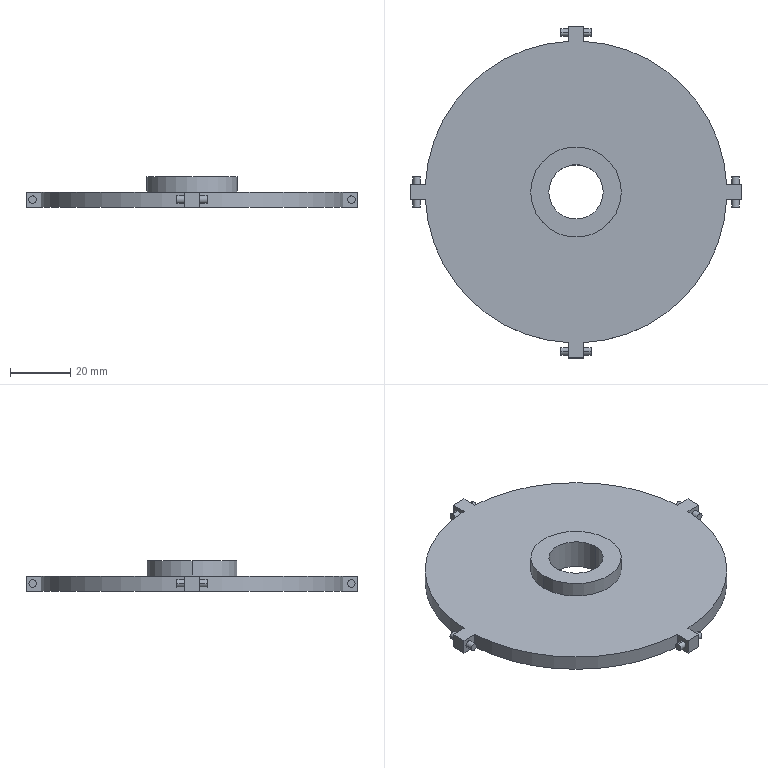Part | SolidWorks | features ICE 4, CirPattern 1, Extrusion 1 | 1 solid | 47 faces | box 110 x 110 x 10 mm | volume 40860 mm3 | cylinder 24 | plane 23 | commonest cylinder face diameters 2.5 x16 100 x4 18 x2 30 x2
STEP:
#1=CARTESIAN_POINT('',(54.05,-5.,2.5));
#2=VERTEX_POINT('',#1);
#3=CARTESIAN_POINT('',(51.55,-5.,2.5));
#4=VERTEX_POINT('',#3);
#5=CARTESIAN_POINT('',(52.8,-5.,2.5));
#6=DIRECTION('',(0.,-1.,0.));
#7=DIRECTION('',(0.,0.,-1.));
#8=AXIS2_PLACEMENT_3D('',#5,#6,#7);
#9=CIRCLE('',#8,1.25);
#10=EDGE_CURVE('',#2,#4,#9,.T.);
#11=ORIENTED_EDGE('',*,*,#10,.F.);
#12=CARTESIAN_POINT('',(54.05,-2.5,2.5));
#13=VERTEX_POINT('',#12);
#14=CARTESIAN_POINT('',(54.05,-5.,2.5));
#15=DIRECTION('',(0.,1.,0.));
#16=VECTOR('',#15,1000.);
#17=LINE('',#14,#16);
#18=EDGE_CURVE('',#2,#13,#17,.T.);
#19=ORIENTED_EDGE('',*,*,#18,.T.);
#20=CARTESIAN_POINT('',(51.55,-2.5,2.5));
#21=VERTEX_POINT('',#20);
#22=CARTESIAN_POINT('',(52.8,-2.5,2.5));
#23=DIRECTION('',(0.,1.,0.));
#24=DIRECTION('',(1.,0.,0.));
#25=AXIS2_PLACEMENT_3D('',#22,#23,#24);
#26=CIRCLE('',#25,1.25);
#27=EDGE_CURVE('',#21,#13,#26,.T.);
#28=ORIENTED_EDGE('',*,*,#27,.F.);
#29=CARTESIAN_POINT('',(51.55,-5.,2.5));
#30=DIRECTION('',(0.,1.,0.));
#31=VECTOR('',#30,1000.);
#32=LINE('',#29,#31);
#33=EDGE_CURVE('',#4,#21,#32,.T.);
#34=ORIENTED_EDGE('',*,*,#33,.F.);
#35=EDGE_LOOP('',(#11,#19,#28,#34));
#36=FACE_OUTER_BOUND('',#35,.T.);
#37=CARTESIAN_POINT('',(52.8,-5.,2.5));
#38=DIRECTION('',(0.,1.,0.));
#39=DIRECTION('',(-1.,0.,0.));
#40=AXIS2_PLACEMENT_3D('',#37,#38,#39);
#41=CYLINDRICAL_SURFACE('',#40,1.25);
#42=ADVANCED_FACE('',(#36),#41,.T.);
#43=CARTESIAN_POINT('',(54.05,2.5,2.5));
#44=VERTEX_POINT('',#43);
#45=CARTESIAN_POINT('',(51.55,2.5,2.5));
#46=VERTEX_POINT('',#45);
#47=CARTESIAN_POINT('',(52.8,2.5,2.5));
#48=DIRECTION('',(0.,-1.,0.));
#49=DIRECTION('',(-1.,0.,0.));
#50=AXIS2_PLACEMENT_3D('',#47,#48,#49);
#51=CIRCLE('',#50,1.25);
#52=EDGE_CURVE('',#44,#46,#51,.T.);
#53=ORIENTED_EDGE('',*,*,#52,.F.);
#54=CARTESIAN_POINT('',(54.05,5.,2.5));
#55=VERTEX_POINT('',#54);
#56=CARTESIAN_POINT('',(54.05,-5.,2.5));
#57=DIRECTION('',(0.,1.,0.));
#58=VECTOR('',#57,1000.);
#59=LINE('',#56,#58);
#60=EDGE_CURVE('',#44,#55,#59,.T.);
#61=ORIENTED_EDGE('',*,*,#60,.T.);
#62=CARTESIAN_POINT('',(51.55,5.,2.5));
#63=VERTEX_POINT('',#62);
#64=CARTESIAN_POINT('',(52.8,5.,2.5));
#65=DIRECTION('',(0.,-1.,0.));
#66=DIRECTION('',(0.,0.,-1.));
#67=AXIS2_PLACEMENT_3D('',#64,#65,#66);
#68=CIRCLE('',#67,1.25);
#69=EDGE_CURVE('',#55,#63,#68,.T.);
#70=ORIENTED_EDGE('',*,*,#69,.T.);
#71=CARTESIAN_POINT('',(51.55,-5.,2.5));
#72=DIRECTION('',(0.,1.,0.));
#73=VECTOR('',#72,1000.);
#74=LINE('',#71,#73);
#75=EDGE_CURVE('',#46,#63,#74,.T.);
#76=ORIENTED_EDGE('',*,*,#75,.F.);
#77=EDGE_LOOP('',(#53,#61,#70,#76));
#78=FACE_OUTER_BOUND('',#77,.T.);
#79=CARTESIAN_POINT('',(52.8,-5.,2.5));
#80=DIRECTION('',(0.,1.,0.));
#81=DIRECTION('',(-1.,0.,0.));
#82=AXIS2_PLACEMENT_3D('',#79,#80,#81);
#83=CYLINDRICAL_SURFACE('',#82,1.25);
#84=ADVANCED_FACE('',(#78),#83,.T.);
#85=CARTESIAN_POINT('',(2.5,-52.8,3.75));
#86=VERTEX_POINT('',#85);
#87=CARTESIAN_POINT('',(2.5,-52.8,1.25));
#88=VERTEX_POINT('',#87);
#89=CARTESIAN_POINT('',(2.5,-52.8,2.5));
#90=DIRECTION('',(-1.,0.,0.));
#91=DIRECTION('',(0.,0.,-1.));
#92=AXIS2_PLACEMENT_3D('',#89,#90,#91);
#93=CIRCLE('',#92,1.25);
#94=EDGE_CURVE('',#86,#88,#93,.T.);
#95=ORIENTED_EDGE('',*,*,#94,.F.);
#96=CARTESIAN_POINT('',(5.,-52.8,3.75));
#97=VERTEX_POINT('',#96);
#98=CARTESIAN_POINT('',(-5.,-52.8,3.75));
#99=DIRECTION('',(1.,0.,0.));
#100=VECTOR('',#99,1000.);
#101=LINE('',#98,#100);
#102=EDGE_CURVE('',#86,#97,#101,.T.);
#103=ORIENTED_EDGE('',*,*,#102,.T.);
#104=CARTESIAN_POINT('',(5.,-52.8,1.25));
#105=VERTEX_POINT('',#104);
#106=CARTESIAN_POINT('',(5.,-52.8,2.5));
#107=DIRECTION('',(-1.,0.,0.));
#108=DIRECTION('',(0.,0.,-1.));
#109=AXIS2_PLACEMENT_3D('',#106,#107,#108);
#110=CIRCLE('',#109,1.25);
#111=EDGE_CURVE('',#97,#105,#110,.T.);
#112=ORIENTED_EDGE('',*,*,#111,.T.);
#113=CARTESIAN_POINT('',(-5.,-52.8,1.25));
#114=DIRECTION('',(1.,0.,0.));
#115=VECTOR('',#114,1000.);
#116=LINE('',#113,#115);
#117=EDGE_CURVE('',#88,#105,#116,.T.);
#118=ORIENTED_EDGE('',*,*,#117,.F.);
#119=EDGE_LOOP('',(#95,#103,#112,#118));
#120=FACE_OUTER_BOUND('',#119,.T.);
#121=CARTESIAN_POINT('',(-5.,-52.8,2.5));
#122=DIRECTION('',(1.,0.,0.));
#123=DIRECTION('',(0.,0.,-1.));
#124=AXIS2_PLACEMENT_3D('',#121,#122,#123);
#125=CYLINDRICAL_SURFACE('',#124,1.25);
#126=ADVANCED_FACE('',(#120),#125,.T.);
#127=CARTESIAN_POINT('',(-5.,-52.8,3.75));
#128=VERTEX_POINT('',#127);
#129=CARTESIAN_POINT('',(-5.,-52.8,1.25));
#130=VERTEX_POINT('',#129);
#131=CARTESIAN_POINT('',(-5.,-52.8,2.5));
#132=DIRECTION('',(-1.,0.,0.));
#133=DIRECTION('',(0.,0.,-1.));
#134=AXIS2_PLACEMENT_3D('',#131,#132,#133);
#135=CIRCLE('',#134,1.25);
#136=EDGE_CURVE('',#128,#130,#135,.T.);
#137=ORIENTED_EDGE('',*,*,#136,.F.);
#138=CARTESIAN_POINT('',(-2.5,-52.8,3.75));
#139=VERTEX_POINT('',#138);
#140=CARTESIAN_POINT('',(-5.,-52.8,3.75));
#141=DIRECTION('',(1.,0.,0.));
#142=VECTOR('',#141,1000.);
#143=LINE('',#140,#142);
#144=EDGE_CURVE('',#128,#139,#143,.T.);
#145=ORIENTED_EDGE('',*,*,#144,.T.);
#146=CARTESIAN_POINT('',(-2.5,-52.8,1.25));
#147=VERTEX_POINT('',#146);
#148=CARTESIAN_POINT('',(-2.5,-52.8,2.5));
#149=DIRECTION('',(1.,0.,0.));
#150=DIRECTION('',(0.,0.,1.));
#151=AXIS2_PLACEMENT_3D('',#148,#149,#150);
#152=CIRCLE('',#151,1.25);
#153=EDGE_CURVE('',#147,#139,#152,.T.);
#154=ORIENTED_EDGE('',*,*,#153,.F.);
#155=CARTESIAN_POINT('',(-5.,-52.8,1.25));
#156=DIRECTION('',(1.,0.,0.));
#157=VECTOR('',#156,1000.);
#158=LINE('',#155,#157);
#159=EDGE_CURVE('',#130,#147,#158,.T.);
#160=ORIENTED_EDGE('',*,*,#159,.F.);
#161=EDGE_LOOP('',(#137,#145,#154,#160));
#162=FACE_OUTER_BOUND('',#161,.T.);
#163=CARTESIAN_POINT('',(-5.,-52.8,2.5));
#164=DIRECTION('',(1.,0.,0.));
#165=DIRECTION('',(0.,0.,-1.));
#166=AXIS2_PLACEMENT_3D('',#163,#164,#165);
#167=CYLINDRICAL_SURFACE('',#166,1.25);
#168=ADVANCED_FACE('',(#162),#167,.T.);
#169=CARTESIAN_POINT('',(-54.05,5.,2.5));
#170=VERTEX_POINT('',#169);
#171=CARTESIAN_POINT('',(-51.55,5.,2.5));
#172=VERTEX_POINT('',#171);
#173=CARTESIAN_POINT('',(-52.8,5.,2.5));
#174=DIRECTION('',(0.,1.,0.));
#175=DIRECTION('',(0.,0.,-1.));
#176=AXIS2_PLACEMENT_3D('',#173,#174,#175);
#177=CIRCLE('',#176,1.25);
#178=EDGE_CURVE('',#170,#172,#177,.T.);
#179=ORIENTED_EDGE('',*,*,#178,.F.);
#180=CARTESIAN_POINT('',(-54.05,2.5,2.5));
#181=VERTEX_POINT('',#180);
#182=CARTESIAN_POINT('',(-54.05,5.,2.5));
#183=DIRECTION('',(0.,-1.,0.));
#184=VECTOR('',#183,1000.);
#185=LINE('',#182,#184);
#186=EDGE_CURVE('',#170,#181,#185,.T.);
#187=ORIENTED_EDGE('',*,*,#186,.T.);
#188=CARTESIAN_POINT('',(-51.55,2.5,2.5));
#189=VERTEX_POINT('',#188);
#190=CARTESIAN_POINT('',(-52.8,2.5,2.5));
#191=DIRECTION('',(0.,-1.,0.));
#192=DIRECTION('',(-1.,0.,0.));
#193=AXIS2_PLACEMENT_3D('',#190,#191,#192);
#194=CIRCLE('',#193,1.25);
#195=EDGE_CURVE('',#189,#181,#194,.T.);
#196=ORIENTED_EDGE('',*,*,#195,.F.);
#197=CARTESIAN_POINT('',(-51.55,5.,2.5));
#198=DIRECTION('',(0.,-1.,0.));
#199=VECTOR('',#198,1000.);
#200=LINE('',#197,#199);
#201=EDGE_CURVE('',#172,#189,#200,.T.);
#202=ORIENTED_EDGE('',*,*,#201,.F.);
#203=EDGE_LOOP('',(#179,#187,#196,#202));
#204=FACE_OUTER_BOUND('',#203,.T.);
#205=CARTESIAN_POINT('',(-52.8,5.,2.5));
#206=DIRECTION('',(0.,-1.,0.));
#207=DIRECTION('',(1.,0.,0.));
#208=AXIS2_PLACEMENT_3D('',#205,#206,#207);
#209=CYLINDRICAL_SURFACE('',#208,1.25);
#210=ADVANCED_FACE('',(#204),#209,.T.);
#211=CARTESIAN_POINT('',(-54.05,-2.5,2.5));
#212=VERTEX_POINT('',#211);
#213=CARTESIAN_POINT('',(-51.55,-2.5,2.5));
#214=VERTEX_POINT('',#213);
#215=CARTESIAN_POINT('',(-52.8,-2.5,2.5));
#216=DIRECTION('',(0.,1.,0.));
#217=DIRECTION('',(1.,0.,0.));
#218=AXIS2_PLACEMENT_3D('',#215,#216,#217);
#219=CIRCLE('',#218,1.25);
#220=EDGE_CURVE('',#212,#214,#219,.T.);
#221=ORIENTED_EDGE('',*,*,#220,.F.);
#222=CARTESIAN_POINT('',(-54.05,-5.,2.5));
#223=VERTEX_POINT('',#222);
#224=CARTESIAN_POINT('',(-54.05,5.,2.5));
#225=DIRECTION('',(0.,-1.,0.));
#226=VECTOR('',#225,1000.);
#227=LINE('',#224,#226);
#228=EDGE_CURVE('',#212,#223,#227,.T.);
#229=ORIENTED_EDGE('',*,*,#228,.T.);
#230=CARTESIAN_POINT('',(-51.55,-5.,2.5));
#231=VERTEX_POINT('',#230);
#232=CARTESIAN_POINT('',(-52.8,-5.,2.5));
#233=DIRECTION('',(0.,1.,0.));
#234=DIRECTION('',(0.,0.,-1.));
#235=AXIS2_PLACEMENT_3D('',#232,#233,#234);
#236=CIRCLE('',#235,1.25);
#237=EDGE_CURVE('',#223,#231,#236,.T.);
#238=ORIENTED_EDGE('',*,*,#237,.T.);
#239=CARTESIAN_POINT('',(-51.55,5.,2.5));
#240=DIRECTION('',(0.,-1.,0.));
#241=VECTOR('',#240,1000.);
#242=LINE('',#239,#241);
#243=EDGE_CURVE('',#214,#231,#242,.T.);
#244=ORIENTED_EDGE('',*,*,#243,.F.);
#245=EDGE_LOOP('',(#221,#229,#238,#244));
#246=FACE_OUTER_BOUND('',#245,.T.);
#247=CARTESIAN_POINT('',(-52.8,5.,2.5));
#248=DIRECTION('',(0.,-1.,0.));
#249=DIRECTION('',(1.,0.,0.));
#250=AXIS2_PLACEMENT_3D('',#247,#248,#249);
#251=CYLINDRICAL_SURFACE('',#250,1.25);
#252=ADVANCED_FACE('',(#246),#251,.T.);
#253=CARTESIAN_POINT('',(5.,52.8,1.25));
#254=VERTEX_POINT('',#253);
#255=CARTESIAN_POINT('',(5.,52.8,3.75));
#256=VERTEX_POINT('',#255);
#257=CARTESIAN_POINT('',(5.,52.8,2.5));
#258=DIRECTION('',(1.,0.,0.));
#259=DIRECTION('',(0.,0.,-1.));
#260=AXIS2_PLACEMENT_3D('',#257,#258,#259);
#261=CIRCLE('',#260,1.25);
#262=EDGE_CURVE('',#254,#256,#261,.T.);
#263=ORIENTED_EDGE('',*,*,#262,.F.);
#264=CARTESIAN_POINT('',(2.5,52.8,1.25));
#265=VERTEX_POINT('',#264);
#266=CARTESIAN_POINT('',(5.,52.8,1.25));
#267=DIRECTION('',(-1.,0.,0.));
#268=VECTOR('',#267,1000.);
#269=LINE('',#266,#268);
#270=EDGE_CURVE('',#254,#265,#269,.T.);
#271=ORIENTED_EDGE('',*,*,#270,.T.);
#272=CARTESIAN_POINT('',(2.5,52.8,3.75));
#273=VERTEX_POINT('',#272);
#274=CARTESIAN_POINT('',(2.5,52.8,2.5));
#275=DIRECTION('',(-1.,0.,0.));
#276=DIRECTION('',(0.,0.,-1.));
#277=AXIS2_PLACEMENT_3D('',#274,#275,#276);
#278=CIRCLE('',#277,1.25);
#279=EDGE_CURVE('',#273,#265,#278,.T.);
#280=ORIENTED_EDGE('',*,*,#279,.F.);
#281=CARTESIAN_POINT('',(5.,52.8,3.75));
#282=DIRECTION('',(-1.,0.,0.));
#283=VECTOR('',#282,1000.);
#284=LINE('',#281,#283);
#285=EDGE_CURVE('',#256,#273,#284,.T.);
#286=ORIENTED_EDGE('',*,*,#285,.F.);
#287=EDGE_LOOP('',(#263,#271,#280,#286));
#288=FACE_OUTER_BOUND('',#287,.T.);
#289=CARTESIAN_POINT('',(5.,52.8,2.5));
#290=DIRECTION('',(-1.,0.,0.));
#291=DIRECTION('',(0.,0.,1.));
#292=AXIS2_PLACEMENT_3D('',#289,#290,#291);
#293=CYLINDRICAL_SURFACE('',#292,1.25);
#294=ADVANCED_FACE('',(#288),#293,.T.);
#295=CARTESIAN_POINT('',(-2.5,52.8,1.25));
#296=VERTEX_POINT('',#295);
#297=CARTESIAN_POINT('',(-2.5,52.8,3.75));
#298=VERTEX_POINT('',#297);
#299=CARTESIAN_POINT('',(-2.5,52.8,2.5));
#300=DIRECTION('',(1.,0.,0.));
#301=DIRECTION('',(0.,0.,1.));
#302=AXIS2_PLACEMENT_3D('',#299,#300,#301);
#303=CIRCLE('',#302,1.25);
#304=EDGE_CURVE('',#296,#298,#303,.T.);
#305=ORIENTED_EDGE('',*,*,#304,.F.);
#306=CARTESIAN_POINT('',(-5.,52.8,1.25));
#307=VERTEX_POINT('',#306);
#308=CARTESIAN_POINT('',(5.,52.8,1.25));
#309=DIRECTION('',(-1.,0.,0.));
#310=VECTOR('',#309,1000.);
#311=LINE('',#308,#310);
#312=EDGE_CURVE('',#296,#307,#311,.T.);
#313=ORIENTED_EDGE('',*,*,#312,.T.);
#314=CARTESIAN_POINT('',(-5.,52.8,3.75));
#315=VERTEX_POINT('',#314);
#316=CARTESIAN_POINT('',(-5.,52.8,2.5));
#317=DIRECTION('',(1.,0.,0.));
#318=DIRECTION('',(0.,0.,-1.));
#319=AXIS2_PLACEMENT_3D('',#316,#317,#318);
#320=CIRCLE('',#319,1.25);
#321=EDGE_CURVE('',#307,#315,#320,.T.);
#322=ORIENTED_EDGE('',*,*,#321,.T.);
#323=CARTESIAN_POINT('',(5.,52.8,3.75));
#324=DIRECTION('',(-1.,0.,0.));
#325=VECTOR('',#324,1000.);
#326=LINE('',#323,#325);
#327=EDGE_CURVE('',#298,#315,#326,.T.);
#328=ORIENTED_EDGE('',*,*,#327,.F.);
#329=EDGE_LOOP('',(#305,#313,#322,#328));
#330=FACE_OUTER_BOUND('',#329,.T.);
#331=CARTESIAN_POINT('',(5.,52.8,2.5));
#332=DIRECTION('',(-1.,0.,0.));
#333=DIRECTION('',(0.,0.,1.));
#334=AXIS2_PLACEMENT_3D('',#331,#332,#333);
#335=CYLINDRICAL_SURFACE('',#334,1.25);
#336=ADVANCED_FACE('',(#330),#335,.T.);
#337=CARTESIAN_POINT('',(-9.,0.,0.));
#338=VERTEX_POINT('',#337);
#339=CARTESIAN_POINT('',(9.,0.,0.));
#340=VERTEX_POINT('',#339);
#341=CARTESIAN_POINT('',(0.,0.,0.));
#342=DIRECTION('',(0.,0.,1.));
#343=DIRECTION('',(1.,0.,0.));
#344=AXIS2_PLACEMENT_3D('',#341,#342,#343);
#345=CIRCLE('',#344,9.);
#346=EDGE_CURVE('',#338,#340,#345,.T.);
#347=ORIENTED_EDGE('',*,*,#346,.F.);
#348=CARTESIAN_POINT('',(-9.,0.,10.));
#349=VERTEX_POINT('',#348);
#350=CARTESIAN_POINT('',(-9.,0.,-5.));
#351=DIRECTION('',(0.,0.,1.));
#352=VECTOR('',#351,1000.);
#353=LINE('',#350,#352);
#354=EDGE_CURVE('',#338,#349,#353,.T.);
#355=ORIENTED_EDGE('',*,*,#354,.T.);
#356=CARTESIAN_POINT('',(9.,0.,10.));
#357=VERTEX_POINT('',#356);
#358=CARTESIAN_POINT('',(0.,0.,10.));
#359=DIRECTION('',(0.,0.,1.));
#360=DIRECTION('',(1.,0.,0.));
#361=AXIS2_PLACEMENT_3D('',#358,#359,#360);
#362=CIRCLE('',#361,9.);
#363=EDGE_CURVE('',#349,#357,#362,.T.);
#364=ORIENTED_EDGE('',*,*,#363,.T.);
#365=CARTESIAN_POINT('',(9.,0.,-5.));
#366=DIRECTION('',(0.,0.,1.));
#367=VECTOR('',#366,1000.);
#368=LINE('',#365,#367);
#369=EDGE_CURVE('',#340,#357,#368,.T.);
#370=ORIENTED_EDGE('',*,*,#369,.F.);
#371=EDGE_LOOP('',(#347,#355,#364,#370));
#372=FACE_OUTER_BOUND('',#371,.T.);
#373=CARTESIAN_POINT('',(0.,0.,-5.));
#374=DIRECTION('',(0.,0.,1.));
#375=DIRECTION('',(1.,0.,0.));
#376=AXIS2_PLACEMENT_3D('',#373,#374,#375);
#377=CYLINDRICAL_SURFACE('',#376,9.);
#378=ADVANCED_FACE('',(#372),#377,.F.);
#379=CARTESIAN_POINT('',(15.,0.,10.));
#380=VERTEX_POINT('',#379);
#381=CARTESIAN_POINT('',(-15.,0.,10.));
#382=VERTEX_POINT('',#381);
#383=CARTESIAN_POINT('',(0.,0.,10.));
#384=DIRECTION('',(0.,0.,1.));
#385=DIRECTION('',(1.,0.,0.));
#386=AXIS2_PLACEMENT_3D('',#383,#384,#385);
#387=CIRCLE('',#386,15.);
#388=EDGE_CURVE('',#380,#382,#387,.T.);
#389=ORIENTED_EDGE('',*,*,#388,.F.);
#390=CARTESIAN_POINT('',(15.,0.,5.));
#391=VERTEX_POINT('',#390);
#392=CARTESIAN_POINT('',(15.,0.,10.));
#393=DIRECTION('',(0.,0.,-1.));
#394=VECTOR('',#393,1000.);
#395=LINE('',#392,#394);
#396=EDGE_CURVE('',#380,#391,#395,.T.);
#397=ORIENTED_EDGE('',*,*,#396,.T.);
#398=CARTESIAN_POINT('',(-15.,0.,5.));
#399=VERTEX_POINT('',#398);
#400=CARTESIAN_POINT('',(0.,0.,5.));
#401=DIRECTION('',(0.,0.,1.));
#402=DIRECTION('',(1.,0.,0.));
#403=AXIS2_PLACEMENT_3D('',#400,#401,#402);
#404=CIRCLE('',#403,15.);
#405=EDGE_CURVE('',#391,#399,#404,.T.);
#406=ORIENTED_EDGE('',*,*,#405,.T.);
#407=CARTESIAN_POINT('',(-15.,0.,10.));
#408=DIRECTION('',(0.,0.,-1.));
#409=VECTOR('',#408,1000.);
#410=LINE('',#407,#409);
#411=EDGE_CURVE('',#382,#399,#410,.T.);
#412=ORIENTED_EDGE('',*,*,#411,.F.);
#413=EDGE_LOOP('',(#389,#397,#406,#412));
#414=FACE_OUTER_BOUND('',#413,.T.);
#415=CARTESIAN_POINT('',(0.,0.,10.));
#416=DIRECTION('',(0.,0.,-1.));
#417=DIRECTION('',(-1.,0.,0.));
#418=AXIS2_PLACEMENT_3D('',#415,#416,#417);
#419=CYLINDRICAL_SURFACE('',#418,15.);
#420=ADVANCED_FACE('',(#414),#419,.T.);
#421=CARTESIAN_POINT('',(2.5,-49.937,0.));
#422=VERTEX_POINT('',#421);
#423=CARTESIAN_POINT('',(49.937,-2.5,0.));
#424=VERTEX_POINT('',#423);
#425=CARTESIAN_POINT('',(0.,0.,0.));
#426=DIRECTION('',(0.,0.,1.));
#427=DIRECTION('',(1.,0.,0.));
#428=AXIS2_PLACEMENT_3D('',#425,#426,#427);
#429=CIRCLE('',#428,50.);
#430=EDGE_CURVE('',#422,#424,#429,.T.);
#431=ORIENTED_EDGE('',*,*,#430,.T.);
#432=CARTESIAN_POINT('',(49.937,-2.5,5.));
#433=VERTEX_POINT('',#432);
#434=CARTESIAN_POINT('',(49.937,-2.5,5.));
#435=DIRECTION('',(0.,0.,-1.));
#436=VECTOR('',#435,1000.);
#437=LINE('',#434,#436);
#438=EDGE_CURVE('',#433,#424,#437,.T.);
#439=ORIENTED_EDGE('',*,*,#438,.F.);
#440=CARTESIAN_POINT('',(2.5,-49.937,5.));
#441=VERTEX_POINT('',#440);
#442=CARTESIAN_POINT('',(0.,0.,5.));
#443=DIRECTION('',(0.,0.,1.));
#444=DIRECTION('',(1.,0.,0.));
#445=AXIS2_PLACEMENT_3D('',#442,#443,#444);
#446=CIRCLE('',#445,50.);
#447=EDGE_CURVE('',#441,#433,#446,.T.);
#448=ORIENTED_EDGE('',*,*,#447,.F.);
#449=CARTESIAN_POINT('',(2.5,-49.937,5.));
#450=DIRECTION('',(0.,0.,1.));
#451=VECTOR('',#450,1000.);
#452=LINE('',#449,#451);
#453=EDGE_CURVE('',#422,#441,#452,.T.);
#454=ORIENTED_EDGE('',*,*,#453,.F.);
#455=EDGE_LOOP('',(#431,#439,#448,#454));
#456=FACE_OUTER_BOUND('',#455,.T.);
#457=CARTESIAN_POINT('',(0.,0.,5.));
#458=DIRECTION('',(0.,0.,-1.));
#459=DIRECTION('',(-1.,0.,0.));
#460=AXIS2_PLACEMENT_3D('',#457,#458,#459);
#461=CYLINDRICAL_SURFACE('',#460,50.);
#462=ADVANCED_FACE('',(#456),#461,.T.);
#463=CARTESIAN_POINT('',(49.937,2.5,5.));
#464=VERTEX_POINT('',#463);
#465=CARTESIAN_POINT('',(2.5,49.937,5.));
#466=VERTEX_POINT('',#465);
#467=CARTESIAN_POINT('',(0.,0.,5.));
#468=DIRECTION('',(0.,0.,1.));
#469=DIRECTION('',(1.,0.,0.));
#470=AXIS2_PLACEMENT_3D('',#467,#468,#469);
#471=CIRCLE('',#470,50.);
#472=EDGE_CURVE('',#464,#466,#471,.T.);
#473=ORIENTED_EDGE('',*,*,#472,.F.);
#474=CARTESIAN_POINT('',(49.937,2.5,0.));
#475=VERTEX_POINT('',#474);
#476=CARTESIAN_POINT('',(49.937,2.5,5.));
#477=DIRECTION('',(0.,0.,1.));
#478=VECTOR('',#477,1000.);
#479=LINE('',#476,#478);
#480=EDGE_CURVE('',#475,#464,#479,.T.);
#481=ORIENTED_EDGE('',*,*,#480,.F.);
#482=CARTESIAN_POINT('',(2.5,49.937,0.));
#483=VERTEX_POINT('',#482);
#484=CARTESIAN_POINT('',(0.,0.,0.));
#485=DIRECTION('',(0.,0.,1.));
#486=DIRECTION('',(1.,0.,0.));
#487=AXIS2_PLACEMENT_3D('',#484,#485,#486);
#488=CIRCLE('',#487,50.);
#489=EDGE_CURVE('',#475,#483,#488,.T.);
#490=ORIENTED_EDGE('',*,*,#489,.T.);
#491=CARTESIAN_POINT('',(2.5,49.937,5.));
#492=DIRECTION('',(0.,0.,-1.));
#493=VECTOR('',#492,1000.);
#494=LINE('',#491,#493);
#495=EDGE_CURVE('',#466,#483,#494,.T.);
#496=ORIENTED_EDGE('',*,*,#495,.F.);
#497=EDGE_LOOP('',(#473,#481,#490,#496));
#498=FACE_OUTER_BOUND('',#497,.T.);
#499=CARTESIAN_POINT('',(0.,0.,5.));
#500=DIRECTION('',(0.,0.,-1.));
#501=DIRECTION('',(-1.,0.,0.));
#502=AXIS2_PLACEMENT_3D('',#499,#500,#501);
#503=CYLINDRICAL_SURFACE('',#502,50.);
#504=ADVANCED_FACE('',(#498),#503,.T.);
#505=CARTESIAN_POINT('',(-2.5,49.937,0.));
#506=VERTEX_POINT('',#505);
#507=CARTESIAN_POINT('',(-49.937,2.5,0.));
#508=VERTEX_POINT('',#507);
#509=CARTESIAN_POINT('',(0.,0.,0.));
#510=DIRECTION('',(0.,0.,1.));
#511=DIRECTION('',(1.,0.,0.));
#512=AXIS2_PLACEMENT_3D('',#509,#510,#511);
#513=CIRCLE('',#512,50.);
#514=EDGE_CURVE('',#506,#508,#513,.T.);
#515=ORIENTED_EDGE('',*,*,#514,.T.);
#516=CARTESIAN_POINT('',(-49.937,2.5,5.));
#517=VERTEX_POINT('',#516);
#518=CARTESIAN_POINT('',(-49.937,2.5,5.));
#519=DIRECTION('',(0.,0.,-1.));
#520=VECTOR('',#519,1000.);
#521=LINE('',#518,#520);
#522=EDGE_CURVE('',#517,#508,#521,.T.);
#523=ORIENTED_EDGE('',*,*,#522,.F.);
#524=CARTESIAN_POINT('',(-2.5,49.937,5.));
#525=VERTEX_POINT('',#524);
#526=CARTESIAN_POINT('',(0.,0.,5.));
#527=DIRECTION('',(0.,0.,1.));
#528=DIRECTION('',(1.,0.,0.));
#529=AXIS2_PLACEMENT_3D('',#526,#527,#528);
#530=CIRCLE('',#529,50.);
#531=EDGE_CURVE('',#525,#517,#530,.T.);
#532=ORIENTED_EDGE('',*,*,#531,.F.);
#533=CARTESIAN_POINT('',(-2.5,49.937,5.));
#534=DIRECTION('',(0.,0.,1.));
#535=VECTOR('',#534,1000.);
#536=LINE('',#533,#535);
#537=EDGE_CURVE('',#506,#525,#536,.T.);
#538=ORIENTED_EDGE('',*,*,#537,.F.);
#539=EDGE_LOOP('',(#515,#523,#532,#538));
#540=FACE_OUTER_BOUND('',#539,.T.);
#541=CARTESIAN_POINT('',(0.,0.,5.));
#542=DIRECTION('',(0.,0.,-1.));
#543=DIRECTION('',(-1.,0.,0.));
#544=AXIS2_PLACEMENT_3D('',#541,#542,#543);
#545=CYLINDRICAL_SURFACE('',#544,50.);
#546=ADVANCED_FACE('',(#540),#545,.T.);
#547=CARTESIAN_POINT('',(-49.937,-2.5,0.));
#548=VERTEX_POINT('',#547);
#549=CARTESIAN_POINT('',(-2.5,-49.937,0.));
#550=VERTEX_POINT('',#549);
#551=CARTESIAN_POINT('',(0.,0.,0.));
#552=DIRECTION('',(0.,0.,1.));
#553=DIRECTION('',(1.,0.,0.));
#554=AXIS2_PLACEMENT_3D('',#551,#552,#553);
#555=CIRCLE('',#554,50.);
#556=EDGE_CURVE('',#548,#550,#555,.T.);
#557=ORIENTED_EDGE('',*,*,#556,.T.);
#558=CARTESIAN_POINT('',(-2.5,-49.937,5.));
#559=VERTEX_POINT('',#558);
#560=CARTESIAN_POINT('',(-2.5,-49.937,5.));
#561=DIRECTION('',(0.,0.,-1.));
#562=VECTOR('',#561,1000.);
#563=LINE('',#560,#562);
#564=EDGE_CURVE('',#559,#550,#563,.T.);
#565=ORIENTED_EDGE('',*,*,#564,.F.);
#566=CARTESIAN_POINT('',(-49.937,-2.5,5.));
#567=VERTEX_POINT('',#566);
#568=CARTESIAN_POINT('',(0.,0.,5.));
#569=DIRECTION('',(0.,0.,1.));
#570=DIRECTION('',(1.,0.,0.));
#571=AXIS2_PLACEMENT_3D('',#568,#569,#570);
#572=CIRCLE('',#571,50.);
#573=EDGE_CURVE('',#567,#559,#572,.T.);
#574=ORIENTED_EDGE('',*,*,#573,.F.);
#575=CARTESIAN_POINT('',(-49.937,-2.5,5.));
#576=DIRECTION('',(0.,0.,1.));
#577=VECTOR('',#576,1000.);
#578=LINE('',#575,#577);
#579=EDGE_CURVE('',#548,#567,#578,.T.);
#580=ORIENTED_EDGE('',*,*,#579,.F.);
#581=EDGE_LOOP('',(#557,#565,#574,#580));
#582=FACE_OUTER_BOUND('',#581,.T.);
#583=CARTESIAN_POINT('',(0.,0.,5.));
#584=DIRECTION('',(0.,0.,-1.));
#585=DIRECTION('',(-1.,0.,0.));
#586=AXIS2_PLACEMENT_3D('',#583,#584,#585);
#587=CYLINDRICAL_SURFACE('',#586,50.);
#588=ADVANCED_FACE('',(#582),#587,.T.);
#589=CARTESIAN_POINT('',(0.,0.,5.));
#590=DIRECTION('',(0.,0.,1.));
#591=DIRECTION('',(1.,0.,0.));
#592=AXIS2_PLACEMENT_3D('',#589,#590,#591);
#593=CIRCLE('',#592,15.);
#594=EDGE_CURVE('',#399,#391,#593,.T.);
#595=ORIENTED_EDGE('',*,*,#594,.F.);
#596=ORIENTED_EDGE('',*,*,#405,.F.);
#597=EDGE_LOOP('',(#595,#596));
#598=FACE_BOUND('',#597,.T.);
#599=ORIENTED_EDGE('',*,*,#531,.T.);
#600=CARTESIAN_POINT('',(-55.,2.5,5.));
#601=VERTEX_POINT('',#600);
#602=CARTESIAN_POINT('',(50.001,2.5,5.));
#603=DIRECTION('',(-1.,0.,0.));
#604=VECTOR('',#603,1000.);
#605=LINE('',#602,#604);
#606=EDGE_CURVE('',#517,#601,#605,.T.);
#607=ORIENTED_EDGE('',*,*,#606,.T.);
#608=CARTESIAN_POINT('',(-55.,-2.5,5.));
#609=VERTEX_POINT('',#608);
#610=CARTESIAN_POINT('',(-55.,2.5,5.));
#611=DIRECTION('',(0.,1.,0.));
#612=VECTOR('',#611,1000.);
#613=LINE('',#610,#612);
#614=EDGE_CURVE('',#609,#601,#613,.T.);
#615=ORIENTED_EDGE('',*,*,#614,.F.);
#616=CARTESIAN_POINT('',(50.001,-2.5,5.));
#617=DIRECTION('',(-1.,0.,0.));
#618=VECTOR('',#617,1000.);
#619=LINE('',#616,#618);
#620=EDGE_CURVE('',#567,#609,#619,.T.);
#621=ORIENTED_EDGE('',*,*,#620,.F.);
#622=ORIENTED_EDGE('',*,*,#573,.T.);
#623=CARTESIAN_POINT('',(-2.5,-55.,5.));
#624=VERTEX_POINT('',#623);
#625=CARTESIAN_POINT('',(-2.5,55.001,5.));
#626=DIRECTION('',(0.,-1.,0.));
#627=VECTOR('',#626,1000.);
#628=LINE('',#625,#627);
#629=EDGE_CURVE('',#559,#624,#628,.T.);
#630=ORIENTED_EDGE('',*,*,#629,.T.);
#631=CARTESIAN_POINT('',(2.5,-55.,5.));
#632=VERTEX_POINT('',#631);
#633=CARTESIAN_POINT('',(-2.5,-55.,5.));
#634=DIRECTION('',(-1.,0.,0.));
#635=VECTOR('',#634,1000.);
#636=LINE('',#633,#635);
#637=EDGE_CURVE('',#632,#624,#636,.T.);
#638=ORIENTED_EDGE('',*,*,#637,.F.);
#639=CARTESIAN_POINT('',(2.5,55.001,5.));
#640=DIRECTION('',(0.,-1.,0.));
#641=VECTOR('',#640,1000.);
#642=LINE('',#639,#641);
#643=EDGE_CURVE('',#441,#632,#642,.T.);
#644=ORIENTED_EDGE('',*,*,#643,.F.);
#645=ORIENTED_EDGE('',*,*,#447,.T.);
#646=CARTESIAN_POINT('',(55.,-2.5,5.));
#647=VERTEX_POINT('',#646);
#648=CARTESIAN_POINT('',(-50.001,-2.5,5.));
#649=DIRECTION('',(1.,0.,0.));
#650=VECTOR('',#649,1000.);
#651=LINE('',#648,#650);
#652=EDGE_CURVE('',#433,#647,#651,.T.);
#653=ORIENTED_EDGE('',*,*,#652,.T.);
#654=CARTESIAN_POINT('',(55.,2.5,5.));
#655=VERTEX_POINT('',#654);
#656=CARTESIAN_POINT('',(55.,-2.5,5.));
#657=DIRECTION('',(0.,-1.,0.));
#658=VECTOR('',#657,1000.);
#659=LINE('',#656,#658);
#660=EDGE_CURVE('',#655,#647,#659,.T.);
#661=ORIENTED_EDGE('',*,*,#660,.F.);
#662=CARTESIAN_POINT('',(-50.001,2.5,5.));
#663=DIRECTION('',(1.,0.,0.));
#664=VECTOR('',#663,1000.);
#665=LINE('',#662,#664);
#666=EDGE_CURVE('',#464,#655,#665,.T.);
#667=ORIENTED_EDGE('',*,*,#666,.F.);
#668=ORIENTED_EDGE('',*,*,#472,.T.);
#669=CARTESIAN_POINT('',(2.5,55.,5.));
#670=VERTEX_POINT('',#669);
#671=CARTESIAN_POINT('',(2.5,-50.001,5.));
#672=DIRECTION('',(0.,1.,0.));
#673=VECTOR('',#672,1000.);
#674=LINE('',#671,#673);
#675=EDGE_CURVE('',#466,#670,#674,.T.);
#676=ORIENTED_EDGE('',*,*,#675,.T.);
#677=CARTESIAN_POINT('',(-2.5,55.,5.));
#678=VERTEX_POINT('',#677);
#679=CARTESIAN_POINT('',(2.5,55.,5.));
#680=DIRECTION('',(1.,0.,0.));
#681=VECTOR('',#680,1000.);
#682=LINE('',#679,#681);
#683=EDGE_CURVE('',#678,#670,#682,.T.);
#684=ORIENTED_EDGE('',*,*,#683,.F.);
#685=CARTESIAN_POINT('',(-2.5,-50.001,5.));
#686=DIRECTION('',(0.,1.,0.));
#687=VECTOR('',#686,1000.);
#688=LINE('',#685,#687);
#689=EDGE_CURVE('',#525,#678,#688,.T.);
#690=ORIENTED_EDGE('',*,*,#689,.F.);
#691=EDGE_LOOP('',(#599,#607,#615,#621,#622,#630,#638,#644,#645,#653,#661,#667,#668,#676,#684,#690));
#692=FACE_OUTER_BOUND('',#691,.T.);
#693=CARTESIAN_POINT('',(0.,0.,5.));
#694=DIRECTION('',(0.,0.,1.));
#695=DIRECTION('',(1.,0.,0.));
#696=AXIS2_PLACEMENT_3D('',#693,#694,#695);
#697=PLANE('',#696);
#698=ADVANCED_FACE('',(#598,#692),#697,.T.);
#699=CARTESIAN_POINT('',(0.,0.,0.));
#700=DIRECTION('',(0.,0.,1.));
#701=DIRECTION('',(1.,0.,0.));
#702=AXIS2_PLACEMENT_3D('',#699,#700,#701);
#703=CIRCLE('',#702,9.);
#704=EDGE_CURVE('',#340,#338,#703,.T.);
#705=ORIENTED_EDGE('',*,*,#704,.T.);
#706=ORIENTED_EDGE('',*,*,#346,.T.);
#707=EDGE_LOOP('',(#705,#706));
#708=FACE_BOUND('',#707,.T.);
#709=ORIENTED_EDGE('',*,*,#514,.F.);
#710=CARTESIAN_POINT('',(-2.5,55.,0.));
#711=VERTEX_POINT('',#710);
#712=CARTESIAN_POINT('',(-2.5,-50.001,0.));
#713=DIRECTION('',(0.,1.,0.));
#714=VECTOR('',#713,1000.);
#715=LINE('',#712,#714);
#716=EDGE_CURVE('',#506,#711,#715,.T.);
#717=ORIENTED_EDGE('',*,*,#716,.T.);
#718=CARTESIAN_POINT('',(2.5,55.,0.));
#719=VERTEX_POINT('',#718);
#720=CARTESIAN_POINT('',(0.,55.,0.));
#721=DIRECTION('',(-1.,0.,0.));
#722=VECTOR('',#721,1000.);
#723=LINE('',#720,#722);
#724=EDGE_CURVE('',#719,#711,#723,.T.);
#725=ORIENTED_EDGE('',*,*,#724,.F.);
#726=CARTESIAN_POINT('',(2.5,-50.001,0.));
#727=DIRECTION('',(0.,1.,0.));
#728=VECTOR('',#727,1000.);
#729=LINE('',#726,#728);
#730=EDGE_CURVE('',#483,#719,#729,.T.);
#731=ORIENTED_EDGE('',*,*,#730,.F.);
#732=ORIENTED_EDGE('',*,*,#489,.F.);
#733=CARTESIAN_POINT('',(55.,2.5,0.));
#734=VERTEX_POINT('',#733);
#735=CARTESIAN_POINT('',(-50.001,2.5,0.));
#736=DIRECTION('',(1.,0.,0.));
#737=VECTOR('',#736,1000.);
#738=LINE('',#735,#737);
#739=EDGE_CURVE('',#475,#734,#738,.T.);
#740=ORIENTED_EDGE('',*,*,#739,.T.);
#741=CARTESIAN_POINT('',(55.,-2.5,0.));
#742=VERTEX_POINT('',#741);
#743=CARTESIAN_POINT('',(55.,0.,0.));
#744=DIRECTION('',(0.,1.,0.));
#745=VECTOR('',#744,1000.);
#746=LINE('',#743,#745);
#747=EDGE_CURVE('',#742,#734,#746,.T.);
#748=ORIENTED_EDGE('',*,*,#747,.F.);
#749=CARTESIAN_POINT('',(-50.001,-2.5,0.));
#750=DIRECTION('',(1.,0.,0.));
#751=VECTOR('',#750,1000.);
#752=LINE('',#749,#751);
#753=EDGE_CURVE('',#424,#742,#752,.T.);
#754=ORIENTED_EDGE('',*,*,#753,.F.);
#755=ORIENTED_EDGE('',*,*,#430,.F.);
#756=CARTESIAN_POINT('',(2.5,-55.,0.));
#757=VERTEX_POINT('',#756);
#758=CARTESIAN_POINT('',(2.5,55.001,0.));
#759=DIRECTION('',(0.,-1.,0.));
#760=VECTOR('',#759,1000.);
#761=LINE('',#758,#760);
#762=EDGE_CURVE('',#422,#757,#761,.T.);
#763=ORIENTED_EDGE('',*,*,#762,.T.);
#764=CARTESIAN_POINT('',(-2.5,-55.,0.));
#765=VERTEX_POINT('',#764);
#766=CARTESIAN_POINT('',(0.,-55.,0.));
#767=DIRECTION('',(1.,0.,0.));
#768=VECTOR('',#767,1000.);
#769=LINE('',#766,#768);
#770=EDGE_CURVE('',#765,#757,#769,.T.);
#771=ORIENTED_EDGE('',*,*,#770,.F.);
#772=CARTESIAN_POINT('',(-2.5,55.001,0.));
#773=DIRECTION('',(0.,-1.,0.));
#774=VECTOR('',#773,1000.);
#775=LINE('',#772,#774);
#776=EDGE_CURVE('',#550,#765,#775,.T.);
#777=ORIENTED_EDGE('',*,*,#776,.F.);
#778=ORIENTED_EDGE('',*,*,#556,.F.);
#779=CARTESIAN_POINT('',(-55.,-2.5,0.));
#780=VERTEX_POINT('',#779);
#781=CARTESIAN_POINT('',(50.001,-2.5,0.));
#782=DIRECTION('',(-1.,0.,0.));
#783=VECTOR('',#782,1000.);
#784=LINE('',#781,#783);
#785=EDGE_CURVE('',#548,#780,#784,.T.);
#786=ORIENTED_EDGE('',*,*,#785,.T.);
#787=CARTESIAN_POINT('',(-55.,2.5,0.));
#788=VERTEX_POINT('',#787);
#789=CARTESIAN_POINT('',(-55.,0.,0.));
#790=DIRECTION('',(0.,-1.,0.));
#791=VECTOR('',#790,1000.);
#792=LINE('',#789,#791);
#793=EDGE_CURVE('',#788,#780,#792,.T.);
#794=ORIENTED_EDGE('',*,*,#793,.F.);
#795=CARTESIAN_POINT('',(50.001,2.5,0.));
#796=DIRECTION('',(-1.,0.,0.));
#797=VECTOR('',#796,1000.);
#798=LINE('',#795,#797);
#799=EDGE_CURVE('',#508,#788,#798,.T.);
#800=ORIENTED_EDGE('',*,*,#799,.F.);
#801=EDGE_LOOP('',(#709,#717,#725,#731,#732,#740,#748,#754,#755,#763,#771,#777,#778,#786,#794,#800));
#802=FACE_OUTER_BOUND('',#801,.T.);
#803=CARTESIAN_POINT('',(0.,0.,0.));
#804=DIRECTION('',(0.,0.,1.));
#805=DIRECTION('',(1.,0.,0.));
#806=AXIS2_PLACEMENT_3D('',#803,#804,#805);
#807=PLANE('',#806);
#808=ADVANCED_FACE('',(#708,#802),#807,.F.);
#809=ORIENTED_EDGE('',*,*,#396,.F.);
#810=CARTESIAN_POINT('',(0.,0.,10.));
#811=DIRECTION('',(0.,0.,1.));
#812=DIRECTION('',(1.,0.,0.));
#813=AXIS2_PLACEMENT_3D('',#810,#811,#812);
#814=CIRCLE('',#813,15.);
#815=EDGE_CURVE('',#382,#380,#814,.T.);
#816=ORIENTED_EDGE('',*,*,#815,.F.);
#817=ORIENTED_EDGE('',*,*,#411,.T.);
#818=ORIENTED_EDGE('',*,*,#594,.T.);
#819=EDGE_LOOP('',(#809,#816,#817,#818));
#820=FACE_OUTER_BOUND('',#819,.T.);
#821=CARTESIAN_POINT('',(0.,0.,10.));
#822=DIRECTION('',(0.,0.,-1.));
#823=DIRECTION('',(-1.,0.,0.));
#824=AXIS2_PLACEMENT_3D('',#821,#822,#823);
#825=CYLINDRICAL_SURFACE('',#824,15.);
#826=ADVANCED_FACE('',(#820),#825,.T.);
#827=CARTESIAN_POINT('',(0.,0.,10.));
#828=DIRECTION('',(0.,0.,1.));
#829=DIRECTION('',(1.,0.,0.));
#830=AXIS2_PLACEMENT_3D('',#827,#828,#829);
#831=CIRCLE('',#830,9.);
#832=EDGE_CURVE('',#357,#349,#831,.T.);
#833=ORIENTED_EDGE('',*,*,#832,.F.);
#834=ORIENTED_EDGE('',*,*,#363,.F.);
#835=EDGE_LOOP('',(#833,#834));
#836=FACE_BOUND('',#835,.T.);
#837=ORIENTED_EDGE('',*,*,#815,.T.);
#838=ORIENTED_EDGE('',*,*,#388,.T.);
#839=EDGE_LOOP('',(#837,#838));
#840=FACE_OUTER_BOUND('',#839,.T.);
#841=CARTESIAN_POINT('',(0.,0.,10.));
#842=DIRECTION('',(0.,0.,1.));
#843=DIRECTION('',(1.,0.,0.));
#844=AXIS2_PLACEMENT_3D('',#841,#842,#843);
#845=PLANE('',#844);
#846=ADVANCED_FACE('',(#836,#840),#845,.T.);
#847=ORIENTED_EDGE('',*,*,#354,.F.);
#848=ORIENTED_EDGE('',*,*,#704,.F.);
#849=ORIENTED_EDGE('',*,*,#369,.T.);
#850=ORIENTED_EDGE('',*,*,#832,.T.);
#851=EDGE_LOOP('',(#847,#848,#849,#850));
#852=FACE_OUTER_BOUND('',#851,.T.);
#853=CARTESIAN_POINT('',(0.,0.,-5.));
#854=DIRECTION('',(0.,0.,1.));
#855=DIRECTION('',(1.,0.,0.));
#856=AXIS2_PLACEMENT_3D('',#853,#854,#855);
#857=CYLINDRICAL_SURFACE('',#856,9.);
#858=ADVANCED_FACE('',(#852),#857,.F.);
#859=ORIENTED_EDGE('',*,*,#279,.T.);
#860=CARTESIAN_POINT('',(2.5,52.8,2.5));
#861=DIRECTION('',(-1.,0.,0.));
#862=DIRECTION('',(0.,0.,-1.));
#863=AXIS2_PLACEMENT_3D('',#860,#861,#862);
#864=CIRCLE('',#863,1.25);
#865=EDGE_CURVE('',#265,#273,#864,.T.);
#866=ORIENTED_EDGE('',*,*,#865,.T.);
#867=EDGE_LOOP('',(#859,#866));
#868=FACE_BOUND('',#867,.T.);
#869=ORIENTED_EDGE('',*,*,#675,.F.);
#870=ORIENTED_EDGE('',*,*,#495,.T.);
#871=ORIENTED_EDGE('',*,*,#730,.T.);
#872=CARTESIAN_POINT('',(2.5,55.,0.));
#873=DIRECTION('',(0.,0.,-1.));
#874=VECTOR('',#873,1000.);
#875=LINE('',#872,#874);
#876=EDGE_CURVE('',#670,#719,#875,.T.);
#877=ORIENTED_EDGE('',*,*,#876,.F.);
#878=EDGE_LOOP('',(#869,#870,#871,#877));
#879=FACE_OUTER_BOUND('',#878,.T.);
#880=CARTESIAN_POINT('',(2.5,-50.001,0.));
#881=DIRECTION('',(1.,0.,0.));
#882=DIRECTION('',(0.,0.,-1.));
#883=AXIS2_PLACEMENT_3D('',#880,#881,#882);
#884=PLANE('',#883);
#885=ADVANCED_FACE('',(#868,#879),#884,.T.);
#886=CARTESIAN_POINT('',(-2.5,52.8,2.5));
#887=DIRECTION('',(1.,0.,0.));
#888=DIRECTION('',(0.,0.,1.));
#889=AXIS2_PLACEMENT_3D('',#886,#887,#888);
#890=CIRCLE('',#889,1.25);
#891=EDGE_CURVE('',#298,#296,#890,.T.);
#892=ORIENTED_EDGE('',*,*,#891,.T.);
#893=ORIENTED_EDGE('',*,*,#304,.T.);
#894=EDGE_LOOP('',(#892,#893));
#895=FACE_BOUND('',#894,.T.);
#896=ORIENTED_EDGE('',*,*,#716,.F.);
#897=ORIENTED_EDGE('',*,*,#537,.T.);
#898=ORIENTED_EDGE('',*,*,#689,.T.);
#899=CARTESIAN_POINT('',(-2.5,55.,5.));
#900=DIRECTION('',(0.,0.,1.));
#901=VECTOR('',#900,1000.);
#902=LINE('',#899,#901);
#903=EDGE_CURVE('',#711,#678,#902,.T.);
#904=ORIENTED_EDGE('',*,*,#903,.F.);
#905=EDGE_LOOP('',(#896,#897,#898,#904));
#906=FACE_OUTER_BOUND('',#905,.T.);
#907=CARTESIAN_POINT('',(-2.5,-50.001,5.));
#908=DIRECTION('',(-1.,0.,0.));
#909=DIRECTION('',(0.,0.,1.));
#910=AXIS2_PLACEMENT_3D('',#907,#908,#909);
#911=PLANE('',#910);
#912=ADVANCED_FACE('',(#895,#906),#911,.T.);
#913=ORIENTED_EDGE('',*,*,#724,.T.);
#914=ORIENTED_EDGE('',*,*,#903,.T.);
#915=ORIENTED_EDGE('',*,*,#683,.T.);
#916=ORIENTED_EDGE('',*,*,#876,.T.);
#917=EDGE_LOOP('',(#913,#914,#915,#916));
#918=FACE_OUTER_BOUND('',#917,.T.);
#919=CARTESIAN_POINT('',(0.,55.,0.));
#920=DIRECTION('',(0.,-1.,0.));
#921=DIRECTION('',(0.,0.,-1.));
#922=AXIS2_PLACEMENT_3D('',#919,#920,#921);
#923=PLANE('',#922);
#924=ADVANCED_FACE('',(#918),#923,.F.);
#925=CARTESIAN_POINT('',(-5.,52.8,2.5));
#926=DIRECTION('',(1.,0.,0.));
#927=DIRECTION('',(0.,0.,-1.));
#928=AXIS2_PLACEMENT_3D('',#925,#926,#927);
#929=CIRCLE('',#928,1.25);
#930=EDGE_CURVE('',#315,#307,#929,.T.);
#931=ORIENTED_EDGE('',*,*,#930,.F.);
#932=ORIENTED_EDGE('',*,*,#321,.F.);
#933=EDGE_LOOP('',(#931,#932));
#934=FACE_OUTER_BOUND('',#933,.T.);
#935=CARTESIAN_POINT('',(-5.,52.8,2.5));
#936=DIRECTION('',(1.,0.,0.));
#937=DIRECTION('',(0.,0.,-1.));
#938=AXIS2_PLACEMENT_3D('',#935,#936,#937);
#939=PLANE('',#938);
#940=ADVANCED_FACE('',(#934),#939,.F.);
#941=ORIENTED_EDGE('',*,*,#312,.F.);
#942=ORIENTED_EDGE('',*,*,#891,.F.);
#943=ORIENTED_EDGE('',*,*,#327,.T.);
#944=ORIENTED_EDGE('',*,*,#930,.T.);
#945=EDGE_LOOP('',(#941,#942,#943,#944));
#946=FACE_OUTER_BOUND('',#945,.T.);
#947=CARTESIAN_POINT('',(5.,52.8,2.5));
#948=DIRECTION('',(-1.,0.,0.));
#949=DIRECTION('',(0.,0.,1.));
#950=AXIS2_PLACEMENT_3D('',#947,#948,#949);
#951=CYLINDRICAL_SURFACE('',#950,1.25);
#952=ADVANCED_FACE('',(#946),#951,.T.);
#953=ORIENTED_EDGE('',*,*,#270,.F.);
#954=CARTESIAN_POINT('',(5.,52.8,2.5));
#955=DIRECTION('',(1.,0.,0.));
#956=DIRECTION('',(0.,0.,-1.));
#957=AXIS2_PLACEMENT_3D('',#954,#955,#956);
#958=CIRCLE('',#957,1.25);
#959=EDGE_CURVE('',#256,#254,#958,.T.);
#960=ORIENTED_EDGE('',*,*,#959,.F.);
#961=ORIENTED_EDGE('',*,*,#285,.T.);
#962=ORIENTED_EDGE('',*,*,#865,.F.);
#963=EDGE_LOOP('',(#953,#960,#961,#962));
#964=FACE_OUTER_BOUND('',#963,.T.);
#965=CARTESIAN_POINT('',(5.,52.8,2.5));
#966=DIRECTION('',(-1.,0.,0.));
#967=DIRECTION('',(0.,0.,1.));
#968=AXIS2_PLACEMENT_3D('',#965,#966,#967);
#969=CYLINDRICAL_SURFACE('',#968,1.25);
#970=ADVANCED_FACE('',(#964),#969,.T.);
#971=ORIENTED_EDGE('',*,*,#959,.T.);
#972=ORIENTED_EDGE('',*,*,#262,.T.);
#973=EDGE_LOOP('',(#971,#972));
#974=FACE_OUTER_BOUND('',#973,.T.);
#975=CARTESIAN_POINT('',(5.,52.8,2.5));
#976=DIRECTION('',(1.,0.,0.));
#977=DIRECTION('',(0.,0.,-1.));
#978=AXIS2_PLACEMENT_3D('',#975,#976,#977);
#979=PLANE('',#978);
#980=ADVANCED_FACE('',(#974),#979,.T.);
#981=ORIENTED_EDGE('',*,*,#195,.T.);
#982=CARTESIAN_POINT('',(-52.8,2.5,2.5));
#983=DIRECTION('',(0.,-1.,0.));
#984=DIRECTION('',(-1.,0.,0.));
#985=AXIS2_PLACEMENT_3D('',#982,#983,#984);
#986=CIRCLE('',#985,1.25);
#987=EDGE_CURVE('',#181,#189,#986,.T.);
#988=ORIENTED_EDGE('',*,*,#987,.T.);
#989=EDGE_LOOP('',(#981,#988));
#990=FACE_BOUND('',#989,.T.);
#991=ORIENTED_EDGE('',*,*,#606,.F.);
#992=ORIENTED_EDGE('',*,*,#522,.T.);
#993=ORIENTED_EDGE('',*,*,#799,.T.);
#994=CARTESIAN_POINT('',(-55.,2.5,0.));
#995=DIRECTION('',(0.,0.,-1.));
#996=VECTOR('',#995,1000.);
#997=LINE('',#994,#996);
#998=EDGE_CURVE('',#601,#788,#997,.T.);
#999=ORIENTED_EDGE('',*,*,#998,.F.);
#1000=EDGE_LOOP('',(#991,#992,#993,#999));
#1001=FACE_OUTER_BOUND('',#1000,.T.);
#1002=CARTESIAN_POINT('',(50.001,2.5,0.));
#1003=DIRECTION('',(0.,1.,0.));
#1004=DIRECTION('',(-1.,0.,0.));
#1005=AXIS2_PLACEMENT_3D('',#1002,#1003,#1004);
#1006=PLANE('',#1005);
#1007=ADVANCED_FACE('',(#990,#1001),#1006,.T.);
#1008=CARTESIAN_POINT('',(-52.8,-2.5,2.5));
#1009=DIRECTION('',(0.,1.,0.));
#1010=DIRECTION('',(1.,0.,0.));
#1011=AXIS2_PLACEMENT_3D('',#1008,#1009,#1010);
#1012=CIRCLE('',#1011,1.25);
#1013=EDGE_CURVE('',#214,#212,#1012,.T.);
#1014=ORIENTED_EDGE('',*,*,#1013,.T.);
#1015=ORIENTED_EDGE('',*,*,#220,.T.);
#1016=EDGE_LOOP('',(#1014,#1015));
#1017=FACE_BOUND('',#1016,.T.);
#1018=ORIENTED_EDGE('',*,*,#785,.F.);
#1019=ORIENTED_EDGE('',*,*,#579,.T.);
#1020=ORIENTED_EDGE('',*,*,#620,.T.);
#1021=CARTESIAN_POINT('',(-55.,-2.5,5.));
#1022=DIRECTION('',(0.,0.,1.));
#1023=VECTOR('',#1022,1000.);
#1024=LINE('',#1021,#1023);
#1025=EDGE_CURVE('',#780,#609,#1024,.T.);
#1026=ORIENTED_EDGE('',*,*,#1025,.F.);
#1027=EDGE_LOOP('',(#1018,#1019,#1020,#1026));
#1028=FACE_OUTER_BOUND('',#1027,.T.);
#1029=CARTESIAN_POINT('',(50.001,-2.5,5.));
#1030=DIRECTION('',(0.,-1.,0.));
#1031=DIRECTION('',(1.,0.,0.));
#1032=AXIS2_PLACEMENT_3D('',#1029,#1030,#1031);
#1033=PLANE('',#1032);
#1034=ADVANCED_FACE('',(#1017,#1028),#1033,.T.);
#1035=ORIENTED_EDGE('',*,*,#793,.T.);
#1036=ORIENTED_EDGE('',*,*,#1025,.T.);
#1037=ORIENTED_EDGE('',*,*,#614,.T.);
#1038=ORIENTED_EDGE('',*,*,#998,.T.);
#1039=EDGE_LOOP('',(#1035,#1036,#1037,#1038));
#1040=FACE_OUTER_BOUND('',#1039,.T.);
#1041=CARTESIAN_POINT('',(-55.,0.,0.));
#1042=DIRECTION('',(1.,0.,0.));
#1043=DIRECTION('',(0.,0.,-1.));
#1044=AXIS2_PLACEMENT_3D('',#1041,#1042,#1043);
#1045=PLANE('',#1044);
#1046=ADVANCED_FACE('',(#1040),#1045,.F.);
#1047=ORIENTED_EDGE('',*,*,#770,.T.);
#1048=CARTESIAN_POINT('',(2.5,-55.,5.));
#1049=DIRECTION('',(0.,0.,1.));
#1050=VECTOR('',#1049,1000.);
#1051=LINE('',#1048,#1050);
#1052=EDGE_CURVE('',#757,#632,#1051,.T.);
#1053=ORIENTED_EDGE('',*,*,#1052,.T.);
#1054=ORIENTED_EDGE('',*,*,#637,.T.);
#1055=CARTESIAN_POINT('',(-2.5,-55.,0.));
#1056=DIRECTION('',(0.,0.,-1.));
#1057=VECTOR('',#1056,1000.);
#1058=LINE('',#1055,#1057);
#1059=EDGE_CURVE('',#624,#765,#1058,.T.);
#1060=ORIENTED_EDGE('',*,*,#1059,.T.);
#1061=EDGE_LOOP('',(#1047,#1053,#1054,#1060));
#1062=FACE_OUTER_BOUND('',#1061,.T.);
#1063=CARTESIAN_POINT('',(0.,-55.,0.));
#1064=DIRECTION('',(0.,1.,0.));
#1065=DIRECTION('',(0.,0.,-1.));
#1066=AXIS2_PLACEMENT_3D('',#1063,#1064,#1065);
#1067=PLANE('',#1066);
#1068=ADVANCED_FACE('',(#1062),#1067,.F.);
#1069=CARTESIAN_POINT('',(2.5,-52.8,2.5));
#1070=DIRECTION('',(-1.,0.,0.));
#1071=DIRECTION('',(0.,0.,-1.));
#1072=AXIS2_PLACEMENT_3D('',#1069,#1070,#1071);
#1073=CIRCLE('',#1072,1.25);
#1074=EDGE_CURVE('',#88,#86,#1073,.T.);
#1075=ORIENTED_EDGE('',*,*,#1074,.T.);
#1076=ORIENTED_EDGE('',*,*,#94,.T.);
#1077=EDGE_LOOP('',(#1075,#1076));
#1078=FACE_BOUND('',#1077,.T.);
#1079=ORIENTED_EDGE('',*,*,#762,.F.);
#1080=ORIENTED_EDGE('',*,*,#453,.T.);
#1081=ORIENTED_EDGE('',*,*,#643,.T.);
#1082=ORIENTED_EDGE('',*,*,#1052,.F.);
#1083=EDGE_LOOP('',(#1079,#1080,#1081,#1082));
#1084=FACE_OUTER_BOUND('',#1083,.T.);
#1085=CARTESIAN_POINT('',(2.5,55.001,5.));
#1086=DIRECTION('',(1.,0.,0.));
#1087=DIRECTION('',(0.,0.,-1.));
#1088=AXIS2_PLACEMENT_3D('',#1085,#1086,#1087);
#1089=PLANE('',#1088);
#1090=ADVANCED_FACE('',(#1078,#1084),#1089,.T.);
#1091=ORIENTED_EDGE('',*,*,#153,.T.);
#1092=CARTESIAN_POINT('',(-2.5,-52.8,2.5));
#1093=DIRECTION('',(1.,0.,0.));
#1094=DIRECTION('',(0.,0.,1.));
#1095=AXIS2_PLACEMENT_3D('',#1092,#1093,#1094);
#1096=CIRCLE('',#1095,1.25);
#1097=EDGE_CURVE('',#139,#147,#1096,.T.);
#1098=ORIENTED_EDGE('',*,*,#1097,.T.);
#1099=EDGE_LOOP('',(#1091,#1098));
#1100=FACE_BOUND('',#1099,.T.);
#1101=ORIENTED_EDGE('',*,*,#629,.F.);
#1102=ORIENTED_EDGE('',*,*,#564,.T.);
#1103=ORIENTED_EDGE('',*,*,#776,.T.);
#1104=ORIENTED_EDGE('',*,*,#1059,.F.);
#1105=EDGE_LOOP('',(#1101,#1102,#1103,#1104));
#1106=FACE_OUTER_BOUND('',#1105,.T.);
#1107=CARTESIAN_POINT('',(-2.5,55.001,0.));
#1108=DIRECTION('',(-1.,0.,0.));
#1109=DIRECTION('',(0.,0.,1.));
#1110=AXIS2_PLACEMENT_3D('',#1107,#1108,#1109);
#1111=PLANE('',#1110);
#1112=ADVANCED_FACE('',(#1100,#1106),#1111,.T.);
#1113=ORIENTED_EDGE('',*,*,#27,.T.);
#1114=CARTESIAN_POINT('',(52.8,-2.5,2.5));
#1115=DIRECTION('',(0.,1.,0.));
#1116=DIRECTION('',(1.,0.,0.));
#1117=AXIS2_PLACEMENT_3D('',#1114,#1115,#1116);
#1118=CIRCLE('',#1117,1.25);
#1119=EDGE_CURVE('',#13,#21,#1118,.T.);
#1120=ORIENTED_EDGE('',*,*,#1119,.T.);
#1121=EDGE_LOOP('',(#1113,#1120));
#1122=FACE_BOUND('',#1121,.T.);
#1123=ORIENTED_EDGE('',*,*,#652,.F.);
#1124=ORIENTED_EDGE('',*,*,#438,.T.);
#1125=ORIENTED_EDGE('',*,*,#753,.T.);
#1126=CARTESIAN_POINT('',(55.,-2.5,0.));
#1127=DIRECTION('',(0.,0.,-1.));
#1128=VECTOR('',#1127,1000.);
#1129=LINE('',#1126,#1128);
#1130=EDGE_CURVE('',#647,#742,#1129,.T.);
#1131=ORIENTED_EDGE('',*,*,#1130,.F.);
#1132=EDGE_LOOP('',(#1123,#1124,#1125,#1131));
#1133=FACE_OUTER_BOUND('',#1132,.T.);
#1134=CARTESIAN_POINT('',(-50.001,-2.5,0.));
#1135=DIRECTION('',(0.,-1.,0.));
#1136=DIRECTION('',(1.,0.,0.));
#1137=AXIS2_PLACEMENT_3D('',#1134,#1135,#1136);
#1138=PLANE('',#1137);
#1139=ADVANCED_FACE('',(#1122,#1133),#1138,.T.);
#1140=CARTESIAN_POINT('',(52.8,2.5,2.5));
#1141=DIRECTION('',(0.,-1.,0.));
#1142=DIRECTION('',(-1.,0.,0.));
#1143=AXIS2_PLACEMENT_3D('',#1140,#1141,#1142);
#1144=CIRCLE('',#1143,1.25);
#1145=EDGE_CURVE('',#46,#44,#1144,.T.);
#1146=ORIENTED_EDGE('',*,*,#1145,.T.);
#1147=ORIENTED_EDGE('',*,*,#52,.T.);
#1148=EDGE_LOOP('',(#1146,#1147));
#1149=FACE_BOUND('',#1148,.T.);
#1150=ORIENTED_EDGE('',*,*,#739,.F.);
#1151=ORIENTED_EDGE('',*,*,#480,.T.);
#1152=ORIENTED_EDGE('',*,*,#666,.T.);
#1153=CARTESIAN_POINT('',(55.,2.5,5.));
#1154=DIRECTION('',(0.,0.,1.));
#1155=VECTOR('',#1154,1000.);
#1156=LINE('',#1153,#1155);
#1157=EDGE_CURVE('',#734,#655,#1156,.T.);
#1158=ORIENTED_EDGE('',*,*,#1157,.F.);
#1159=EDGE_LOOP('',(#1150,#1151,#1152,#1158));
#1160=FACE_OUTER_BOUND('',#1159,.T.);
#1161=CARTESIAN_POINT('',(-50.001,2.5,5.));
#1162=DIRECTION('',(0.,1.,0.));
#1163=DIRECTION('',(-1.,0.,0.));
#1164=AXIS2_PLACEMENT_3D('',#1161,#1162,#1163);
#1165=PLANE('',#1164);
#1166=ADVANCED_FACE('',(#1149,#1160),#1165,.T.);
#1167=ORIENTED_EDGE('',*,*,#747,.T.);
#1168=ORIENTED_EDGE('',*,*,#1157,.T.);
#1169=ORIENTED_EDGE('',*,*,#660,.T.);
#1170=ORIENTED_EDGE('',*,*,#1130,.T.);
#1171=EDGE_LOOP('',(#1167,#1168,#1169,#1170));
#1172=FACE_OUTER_BOUND('',#1171,.T.);
#1173=CARTESIAN_POINT('',(55.,0.,0.));
#1174=DIRECTION('',(-1.,0.,0.));
#1175=DIRECTION('',(0.,0.,-1.));
#1176=AXIS2_PLACEMENT_3D('',#1173,#1174,#1175);
#1177=PLANE('',#1176);
#1178=ADVANCED_FACE('',(#1172),#1177,.F.);
#1179=CARTESIAN_POINT('',(-52.8,-5.,2.5));
#1180=DIRECTION('',(0.,1.,0.));
#1181=DIRECTION('',(0.,0.,-1.));
#1182=AXIS2_PLACEMENT_3D('',#1179,#1180,#1181);
#1183=CIRCLE('',#1182,1.25);
#1184=EDGE_CURVE('',#231,#223,#1183,.T.);
#1185=ORIENTED_EDGE('',*,*,#1184,.F.);
#1186=ORIENTED_EDGE('',*,*,#237,.F.);
#1187=EDGE_LOOP('',(#1185,#1186));
#1188=FACE_OUTER_BOUND('',#1187,.T.);
#1189=CARTESIAN_POINT('',(-52.8,-5.,2.5));
#1190=DIRECTION('',(0.,1.,0.));
#1191=DIRECTION('',(0.,0.,-1.));
#1192=AXIS2_PLACEMENT_3D('',#1189,#1190,#1191);
#1193=PLANE('',#1192);
#1194=ADVANCED_FACE('',(#1188),#1193,.F.);
#1195=ORIENTED_EDGE('',*,*,#228,.F.);
#1196=ORIENTED_EDGE('',*,*,#1013,.F.);
#1197=ORIENTED_EDGE('',*,*,#243,.T.);
#1198=ORIENTED_EDGE('',*,*,#1184,.T.);
#1199=EDGE_LOOP('',(#1195,#1196,#1197,#1198));
#1200=FACE_OUTER_BOUND('',#1199,.T.);
#1201=CARTESIAN_POINT('',(-52.8,5.,2.5));
#1202=DIRECTION('',(0.,-1.,0.));
#1203=DIRECTION('',(1.,0.,0.));
#1204=AXIS2_PLACEMENT_3D('',#1201,#1202,#1203);
#1205=CYLINDRICAL_SURFACE('',#1204,1.25);
#1206=ADVANCED_FACE('',(#1200),#1205,.T.);
#1207=ORIENTED_EDGE('',*,*,#186,.F.);
#1208=CARTESIAN_POINT('',(-52.8,5.,2.5));
#1209=DIRECTION('',(0.,1.,0.));
#1210=DIRECTION('',(0.,0.,-1.));
#1211=AXIS2_PLACEMENT_3D('',#1208,#1209,#1210);
#1212=CIRCLE('',#1211,1.25);
#1213=EDGE_CURVE('',#172,#170,#1212,.T.);
#1214=ORIENTED_EDGE('',*,*,#1213,.F.);
#1215=ORIENTED_EDGE('',*,*,#201,.T.);
#1216=ORIENTED_EDGE('',*,*,#987,.F.);
#1217=EDGE_LOOP('',(#1207,#1214,#1215,#1216));
#1218=FACE_OUTER_BOUND('',#1217,.T.);
#1219=CARTESIAN_POINT('',(-52.8,5.,2.5));
#1220=DIRECTION('',(0.,-1.,0.));
#1221=DIRECTION('',(1.,0.,0.));
#1222=AXIS2_PLACEMENT_3D('',#1219,#1220,#1221);
#1223=CYLINDRICAL_SURFACE('',#1222,1.25);
#1224=ADVANCED_FACE('',(#1218),#1223,.T.);
#1225=ORIENTED_EDGE('',*,*,#1213,.T.);
#1226=ORIENTED_EDGE('',*,*,#178,.T.);
#1227=EDGE_LOOP('',(#1225,#1226));
#1228=FACE_OUTER_BOUND('',#1227,.T.);
#1229=CARTESIAN_POINT('',(-52.8,5.,2.5));
#1230=DIRECTION('',(0.,1.,0.));
#1231=DIRECTION('',(0.,0.,-1.));
#1232=AXIS2_PLACEMENT_3D('',#1229,#1230,#1231);
#1233=PLANE('',#1232);
#1234=ADVANCED_FACE('',(#1228),#1233,.T.);
#1235=CARTESIAN_POINT('',(-5.,-52.8,2.5));
#1236=DIRECTION('',(-1.,0.,0.));
#1237=DIRECTION('',(0.,0.,-1.));
#1238=AXIS2_PLACEMENT_3D('',#1235,#1236,#1237);
#1239=CIRCLE('',#1238,1.25);
#1240=EDGE_CURVE('',#130,#128,#1239,.T.);
#1241=ORIENTED_EDGE('',*,*,#1240,.T.);
#1242=ORIENTED_EDGE('',*,*,#136,.T.);
#1243=EDGE_LOOP('',(#1241,#1242));
#1244=FACE_OUTER_BOUND('',#1243,.T.);
#1245=CARTESIAN_POINT('',(-5.,-52.8,2.5));
#1246=DIRECTION('',(-1.,0.,0.));
#1247=DIRECTION('',(0.,0.,-1.));
#1248=AXIS2_PLACEMENT_3D('',#1245,#1246,#1247);
#1249=PLANE('',#1248);
#1250=ADVANCED_FACE('',(#1244),#1249,.T.);
#1251=ORIENTED_EDGE('',*,*,#144,.F.);
#1252=ORIENTED_EDGE('',*,*,#1240,.F.);
#1253=ORIENTED_EDGE('',*,*,#159,.T.);
#1254=ORIENTED_EDGE('',*,*,#1097,.F.);
#1255=EDGE_LOOP('',(#1251,#1252,#1253,#1254));
#1256=FACE_OUTER_BOUND('',#1255,.T.);
#1257=CARTESIAN_POINT('',(-5.,-52.8,2.5));
#1258=DIRECTION('',(1.,0.,0.));
#1259=DIRECTION('',(0.,0.,-1.));
#1260=AXIS2_PLACEMENT_3D('',#1257,#1258,#1259);
#1261=CYLINDRICAL_SURFACE('',#1260,1.25);
#1262=ADVANCED_FACE('',(#1256),#1261,.T.);
#1263=ORIENTED_EDGE('',*,*,#102,.F.);
#1264=ORIENTED_EDGE('',*,*,#1074,.F.);
#1265=ORIENTED_EDGE('',*,*,#117,.T.);
#1266=CARTESIAN_POINT('',(5.,-52.8,2.5));
#1267=DIRECTION('',(-1.,0.,0.));
#1268=DIRECTION('',(0.,0.,-1.));
#1269=AXIS2_PLACEMENT_3D('',#1266,#1267,#1268);
#1270=CIRCLE('',#1269,1.25);
#1271=EDGE_CURVE('',#105,#97,#1270,.T.);
#1272=ORIENTED_EDGE('',*,*,#1271,.T.);
#1273=EDGE_LOOP('',(#1263,#1264,#1265,#1272));
#1274=FACE_OUTER_BOUND('',#1273,.T.);
#1275=CARTESIAN_POINT('',(-5.,-52.8,2.5));
#1276=DIRECTION('',(1.,0.,0.));
#1277=DIRECTION('',(0.,0.,-1.));
#1278=AXIS2_PLACEMENT_3D('',#1275,#1276,#1277);
#1279=CYLINDRICAL_SURFACE('',#1278,1.25);
#1280=ADVANCED_FACE('',(#1274),#1279,.T.);
#1281=ORIENTED_EDGE('',*,*,#1271,.F.);
#1282=ORIENTED_EDGE('',*,*,#111,.F.);
#1283=EDGE_LOOP('',(#1281,#1282));
#1284=FACE_OUTER_BOUND('',#1283,.T.);
#1285=CARTESIAN_POINT('',(5.,-52.8,2.5));
#1286=DIRECTION('',(-1.,0.,0.));
#1287=DIRECTION('',(0.,0.,-1.));
#1288=AXIS2_PLACEMENT_3D('',#1285,#1286,#1287);
#1289=PLANE('',#1288);
#1290=ADVANCED_FACE('',(#1284),#1289,.F.);
#1291=CARTESIAN_POINT('',(52.8,5.,2.5));
#1292=DIRECTION('',(0.,-1.,0.));
#1293=DIRECTION('',(0.,0.,-1.));
#1294=AXIS2_PLACEMENT_3D('',#1291,#1292,#1293);
#1295=CIRCLE('',#1294,1.25);
#1296=EDGE_CURVE('',#63,#55,#1295,.T.);
#1297=ORIENTED_EDGE('',*,*,#1296,.F.);
#1298=ORIENTED_EDGE('',*,*,#69,.F.);
#1299=EDGE_LOOP('',(#1297,#1298));
#1300=FACE_OUTER_BOUND('',#1299,.T.);
#1301=CARTESIAN_POINT('',(52.8,5.,2.5));
#1302=DIRECTION('',(0.,-1.,0.));
#1303=DIRECTION('',(0.,0.,-1.));
#1304=AXIS2_PLACEMENT_3D('',#1301,#1302,#1303);
#1305=PLANE('',#1304);
#1306=ADVANCED_FACE('',(#1300),#1305,.F.);
#1307=ORIENTED_EDGE('',*,*,#60,.F.);
#1308=ORIENTED_EDGE('',*,*,#1145,.F.);
#1309=ORIENTED_EDGE('',*,*,#75,.T.);
#1310=ORIENTED_EDGE('',*,*,#1296,.T.);
#1311=EDGE_LOOP('',(#1307,#1308,#1309,#1310));
#1312=FACE_OUTER_BOUND('',#1311,.T.);
#1313=CARTESIAN_POINT('',(52.8,-5.,2.5));
#1314=DIRECTION('',(0.,1.,0.));
#1315=DIRECTION('',(-1.,0.,0.));
#1316=AXIS2_PLACEMENT_3D('',#1313,#1314,#1315);
#1317=CYLINDRICAL_SURFACE('',#1316,1.25);
#1318=ADVANCED_FACE('',(#1312),#1317,.T.);
#1319=ORIENTED_EDGE('',*,*,#18,.F.);
#1320=CARTESIAN_POINT('',(52.8,-5.,2.5));
#1321=DIRECTION('',(0.,-1.,0.));
#1322=DIRECTION('',(0.,0.,-1.));
#1323=AXIS2_PLACEMENT_3D('',#1320,#1321,#1322);
#1324=CIRCLE('',#1323,1.25);
#1325=EDGE_CURVE('',#4,#2,#1324,.T.);
#1326=ORIENTED_EDGE('',*,*,#1325,.F.);
#1327=ORIENTED_EDGE('',*,*,#33,.T.);
#1328=ORIENTED_EDGE('',*,*,#1119,.F.);
#1329=EDGE_LOOP('',(#1319,#1326,#1327,#1328));
#1330=FACE_OUTER_BOUND('',#1329,.T.);
#1331=CARTESIAN_POINT('',(52.8,-5.,2.5));
#1332=DIRECTION('',(0.,1.,0.));
#1333=DIRECTION('',(-1.,0.,0.));
#1334=AXIS2_PLACEMENT_3D('',#1331,#1332,#1333);
#1335=CYLINDRICAL_SURFACE('',#1334,1.25);
#1336=ADVANCED_FACE('',(#1330),#1335,.T.);
#1337=ORIENTED_EDGE('',*,*,#1325,.T.);
#1338=ORIENTED_EDGE('',*,*,#10,.T.);
#1339=EDGE_LOOP('',(#1337,#1338));
#1340=FACE_OUTER_BOUND('',#1339,.T.);
#1341=CARTESIAN_POINT('',(52.8,-5.,2.5));
#1342=DIRECTION('',(0.,-1.,0.));
#1343=DIRECTION('',(0.,0.,-1.));
#1344=AXIS2_PLACEMENT_3D('',#1341,#1342,#1343);
#1345=PLANE('',#1344);
#1346=ADVANCED_FACE('',(#1340),#1345,.T.);
#1347=CLOSED_SHELL('',(#42,#84,#126,#168,#210,#252,#294,#336,#378,#420,#462,#504,#546,#588,#698,#808,#826,#846,#858,#885,#912,#924,#940,#952,#970,#980,#1007,#1034,#1046,#1068,#1090,#1112,#1139,#1166,#1178,#1194,#1206,#1224,#1234,#1250,#1262,#1280,#1290,#1306,#1318,#1336,#1346));
#1348=MANIFOLD_SOLID_BREP('',#1347);
#1349=CARTESIAN_POINT('',(0.,0.,0.));
#1350=DIRECTION('',(0.,0.,1.));
#1351=DIRECTION('',(1.,0.,0.));
#1352=AXIS2_PLACEMENT_3D('',#1349,#1350,#1351);
#1353=(LENGTH_UNIT()NAMED_UNIT(*)SI_UNIT(.MILLI.,.METRE.));
#1354=UNCERTAINTY_MEASURE_WITH_UNIT(LENGTH_MEASURE(0.00001),#1353,'','');
#1355=(NAMED_UNIT(*)PLANE_ANGLE_UNIT()SI_UNIT($,.RADIAN.));
#1356=(NAMED_UNIT(*)SI_UNIT($,.STERADIAN.)SOLID_ANGLE_UNIT());
#1357=(GEOMETRIC_REPRESENTATION_CONTEXT(3)GLOBAL_UNCERTAINTY_ASSIGNED_CONTEXT((#1354))GLOBAL_UNIT_ASSIGNED_CONTEXT((#1353,#1355,#1356))REPRESENTATION_CONTEXT('',''));
#1358=ADVANCED_BREP_SHAPE_REPRESENTATION('',(#1348,#1352),#1357);